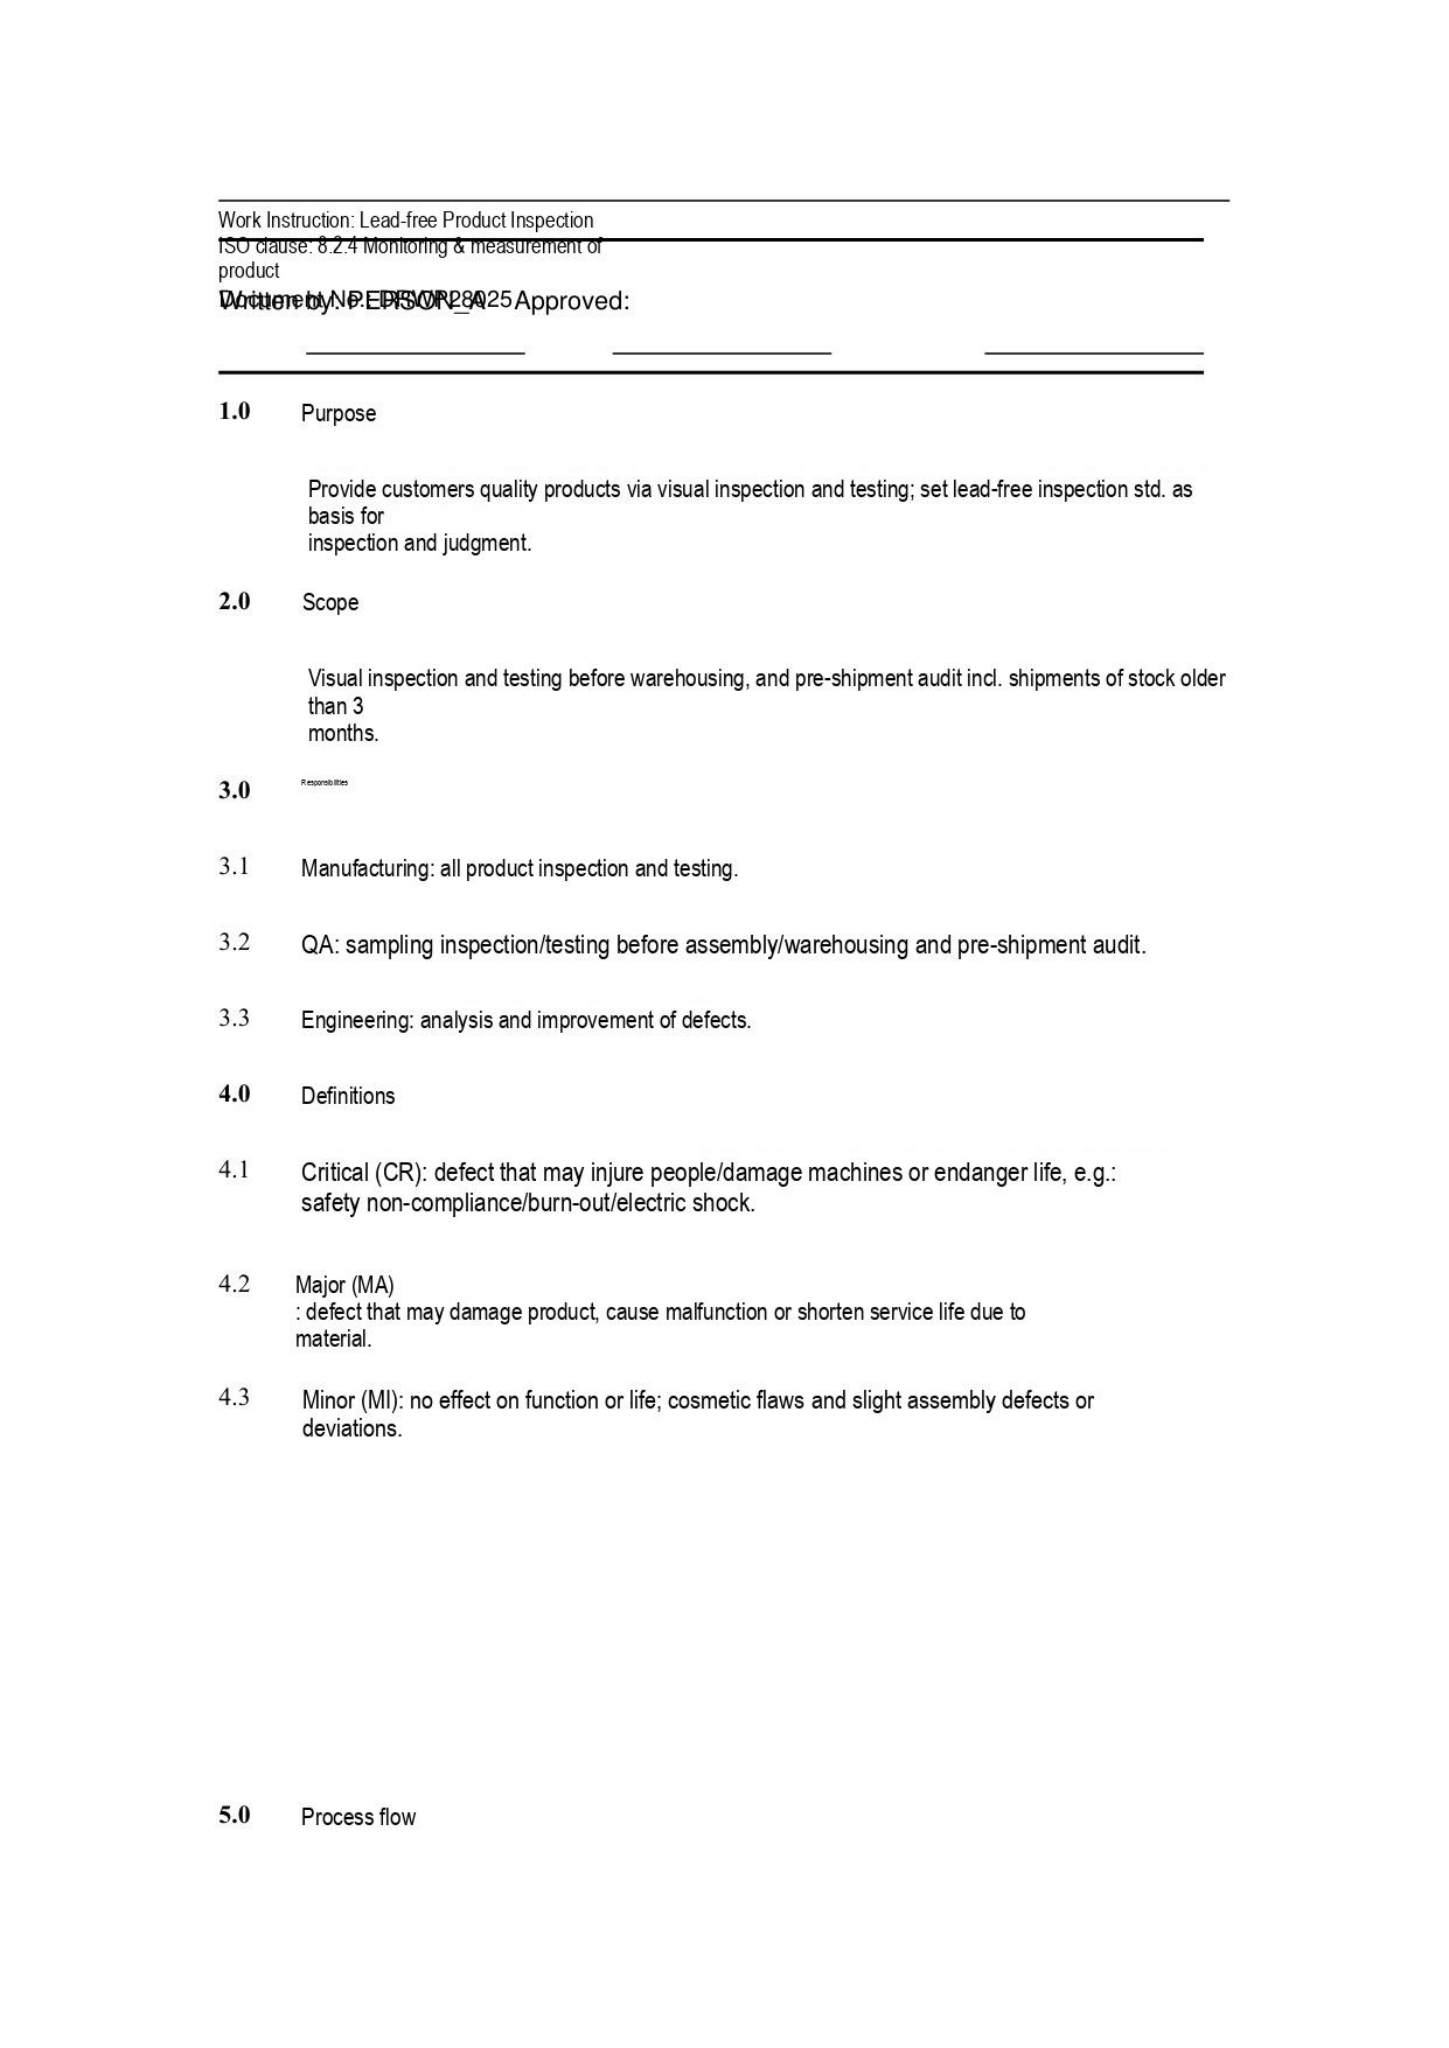Work Instruction: Lead-free Product Inspection
ISO clause: 8.2.4 Monitoring & measurement of product

Written by: PERSON_A Approved:

**1.0** Purpose

Provide customers quality products via visual inspection and testing; set lead-free inspection std. as basis for
inspection and judgment.

**2.0** Scope

Visual inspection and testing before warehousing, and pre-shipment audit incl. shipments of stock older than 3
months.

**3.0** Responsibilities

3.1 Manufacturing: all product inspection and testing.

3.2 QA: sampling inspection/testing before assembly/warehousing and pre-shipment audit.

3.3 Engineering: analysis and improvement of defects.

**4.0** Definitions

4.1 Critical (CR): defect that may injure people/damage machines or endanger life, e.g.:
safety non-compliance/burn-out/electric shock.

4.2 Major (MA)
: defect that may damage product, cause malfunction or shorten service life due to
material.

4.3 Minor (MI): no effect on function or life; cosmetic flaws and slight assembly defects or
deviations.

**5.0** Process flow
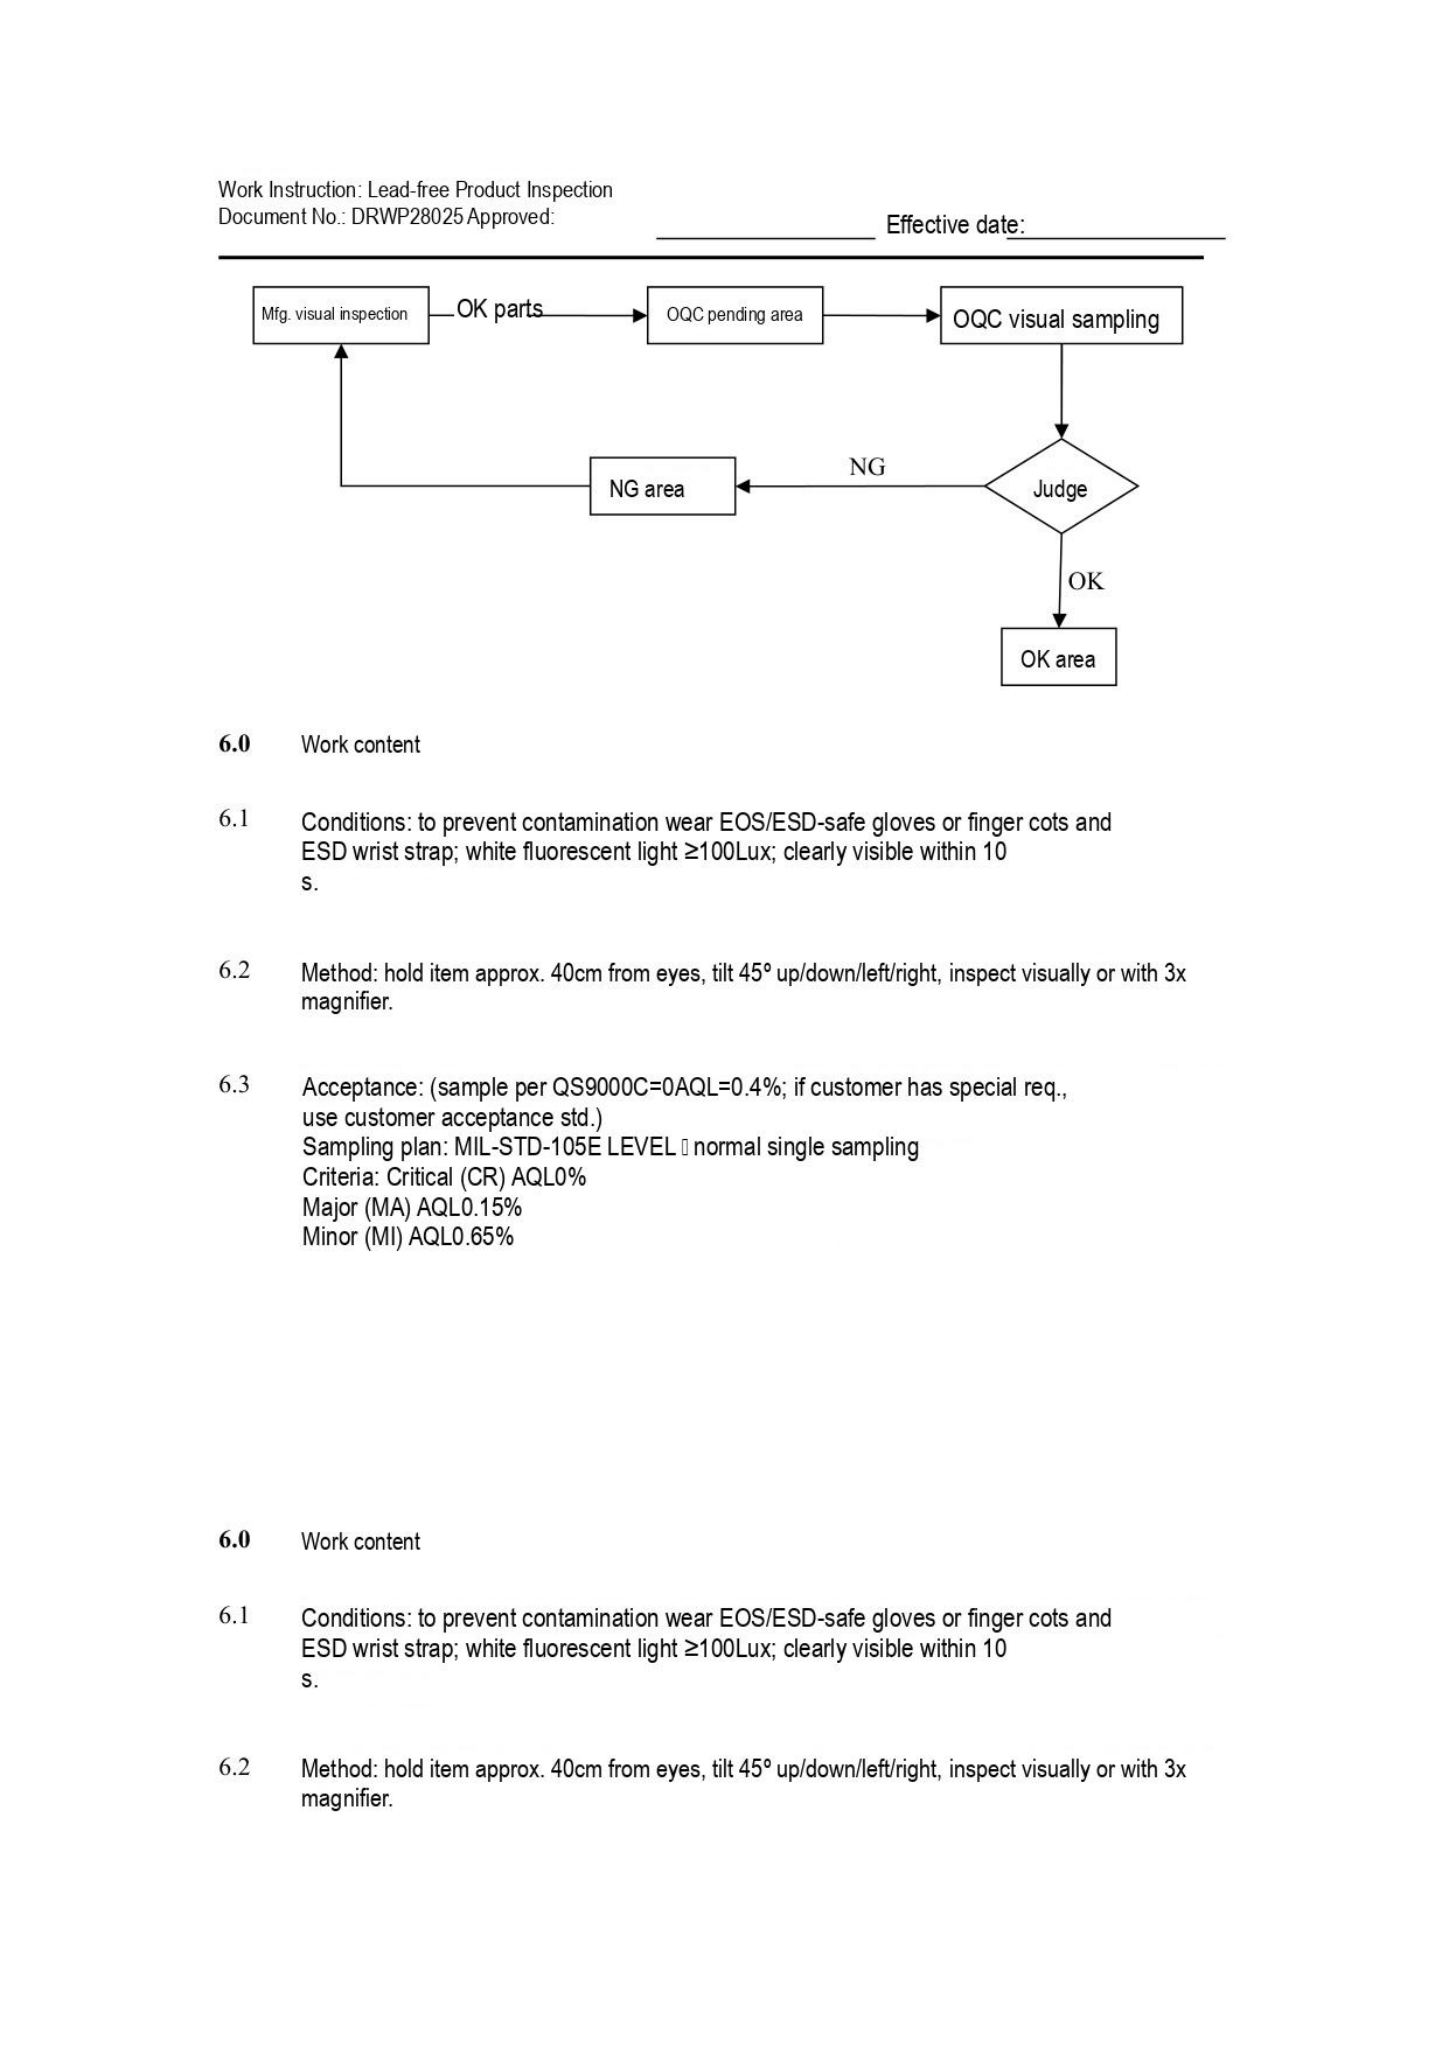Work Instruction: Lead-free Product Inspection
Document No.: DRWP28025 Approved: Effective date:

Mfg. visual inspection
OK parts
OQC pending area
OQC visual sampling
Judge
NG
NG area
OK
OK area

6.0 Work content

6.1 Conditions: to prevent contamination wear EOS/ESD-safe gloves or finger cots and ESD wrist strap; white fluorescent light ≥100Lux; clearly visible within 10 s.

6.2 Method: hold item approx. 40cm from eyes, tilt 45° up/down/left/right, inspect visually or with 3x magnifier.

6.3 Acceptance: (sample per QS9000C=0AQL=0.4%; if customer has special req., use customer acceptance std.)
Sampling plan: MIL-STD-105E LEVEL normal single sampling
Criteria: Critical (CR) AQL0%
Major (MA) AQL0.15%
Minor (MI) AQL0.65%

6.0 Work content

6.1 Conditions: to prevent contamination wear EOS/ESD-safe gloves or finger cots and ESD wrist strap; white fluorescent light ≥100Lux; clearly visible within 10 s.

6.2 Method: hold item approx. 40cm from eyes, tilt 45° up/down/left/right, inspect visually or with 3x magnifier.
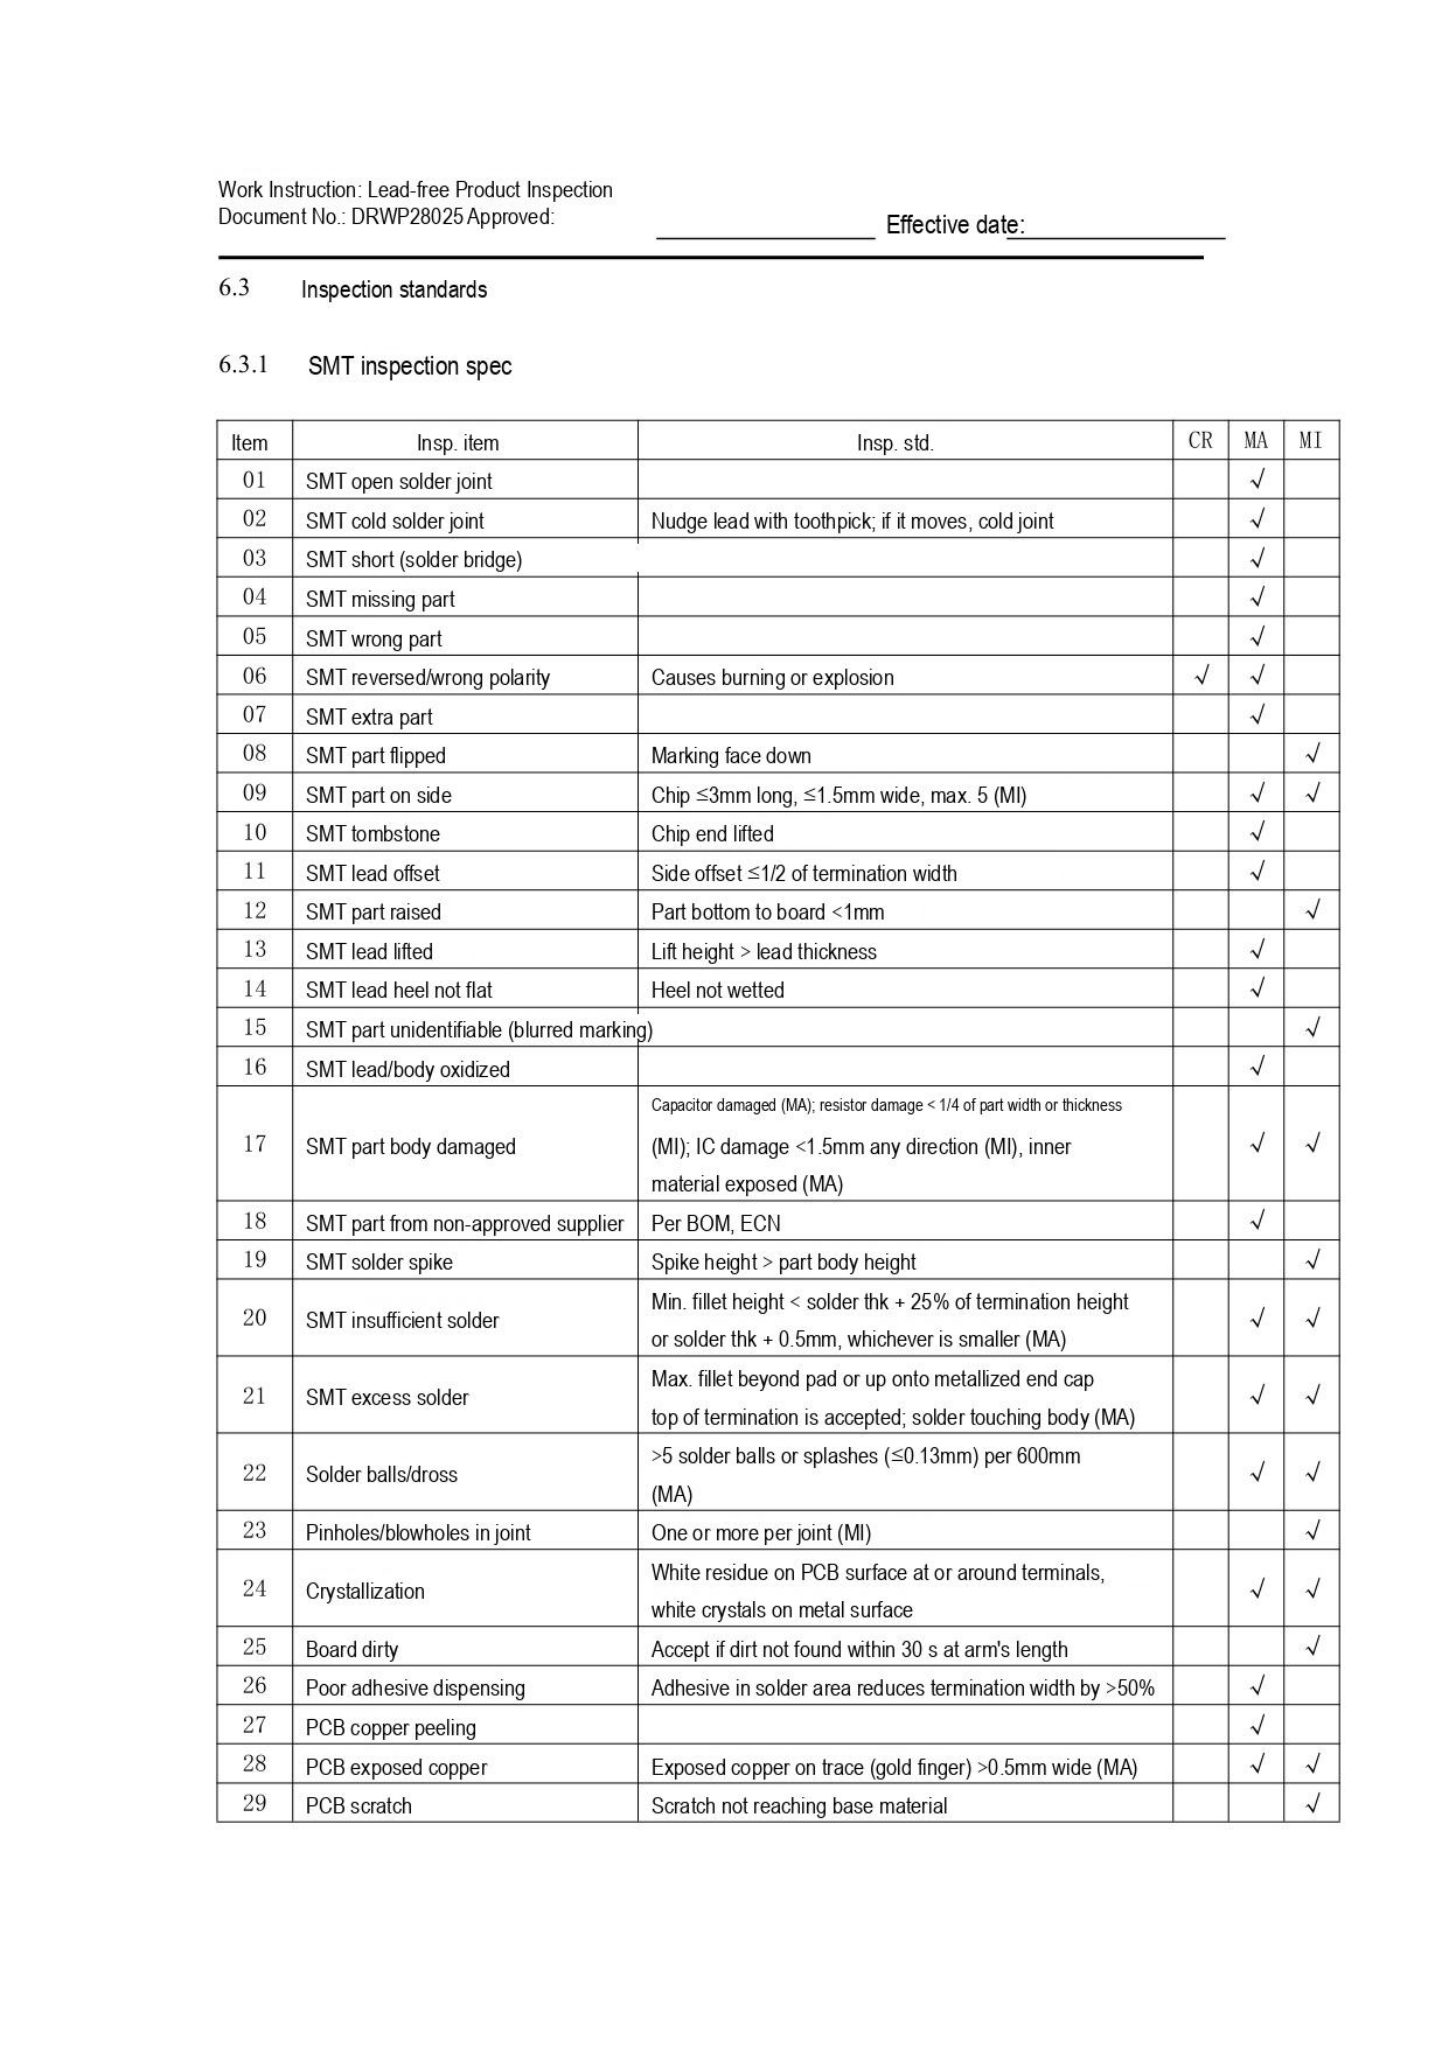Work Instruction: Lead-free Product Inspection
Document No.: DRWP28025 Approved: Effective date:

6.3 Inspection standards

6.3.1 SMT inspection spec

| Item | Insp. item | Insp. std. | CR | MA | MI |
|---|---|---|---|---|---|
| 01 | SMT open solder joint | | | √ | |
| 02 | SMT cold solder joint | Nudge lead with toothpick; if it moves, cold joint | | √ | |
| 03 | SMT short (solder bridge) | | | √ | |
| 04 | SMT missing part | | | √ | |
| 05 | SMT wrong part | | | √ | |
| 06 | SMT reversed/wrong polarity | Causes burning or explosion | √ | √ | |
| 07 | SMT extra part | | | √ | |
| 08 | SMT part flipped | Marking face down | | | √ |
| 09 | SMT part on side | Chip ≤3mm long, ≤1.5mm wide, max. 5 (MI) | | √ | √ |
| 10 | SMT tombstone | Chip end lifted | | √ | |
| 11 | SMT lead offset | Side offset ≤1/2 of termination width | | √ | |
| 12 | SMT part raised | Part bottom to board <1mm | | | √ |
| 13 | SMT lead lifted | Lift height > lead thickness | | √ | |
| 14 | SMT lead heel not flat | Heel not wetted | | √ | |
| 15 | SMT part unidentifiable (blurred marking) | | | | √ |
| 16 | SMT lead/body oxidized | | | √ | |
| 17 | SMT part body damaged | Capacitor damaged (MA); resistor damage < 1/4 of part width or thickness (MI); IC damage <1.5mm any direction (MI), inner material exposed (MA) | | √ | √ |
| 18 | SMT part from non-approved supplier | Per BOM, ECN | | √ | |
| 19 | SMT solder spike | Spike height > part body height | | | √ |
| 20 | SMT insufficient solder | Min. fillet height < solder thk + 25% of termination height or solder thk + 0.5mm, whichever is smaller (MA) | | √ | √ |
| 21 | SMT excess solder | Max. fillet beyond pad or up onto metallized end cap top of termination is accepted; solder touching body (MA) | | √ | √ |
| 22 | Solder balls/dross | >5 solder balls or splashes (≤0.13mm) per 600mm (MA) | | √ | √ |
| 23 | Pinholes/blowholes in joint | One or more per joint (MI) | | | √ |
| 24 | Crystallization | White residue on PCB surface at or around terminals, white crystals on metal surface | | √ | √ |
| 25 | Board dirty | Accept if dirt not found within 30 s at arm's length | | | √ |
| 26 | Poor adhesive dispensing | Adhesive in solder area reduces termination width by >50% | | √ | |
| 27 | PCB copper peeling | | | √ | |
| 28 | PCB exposed copper | Exposed copper on trace (gold finger) >0.5mm wide (MA) | | √ | √ |
| 29 | PCB scratch | Scratch not reaching base material | | | √ |
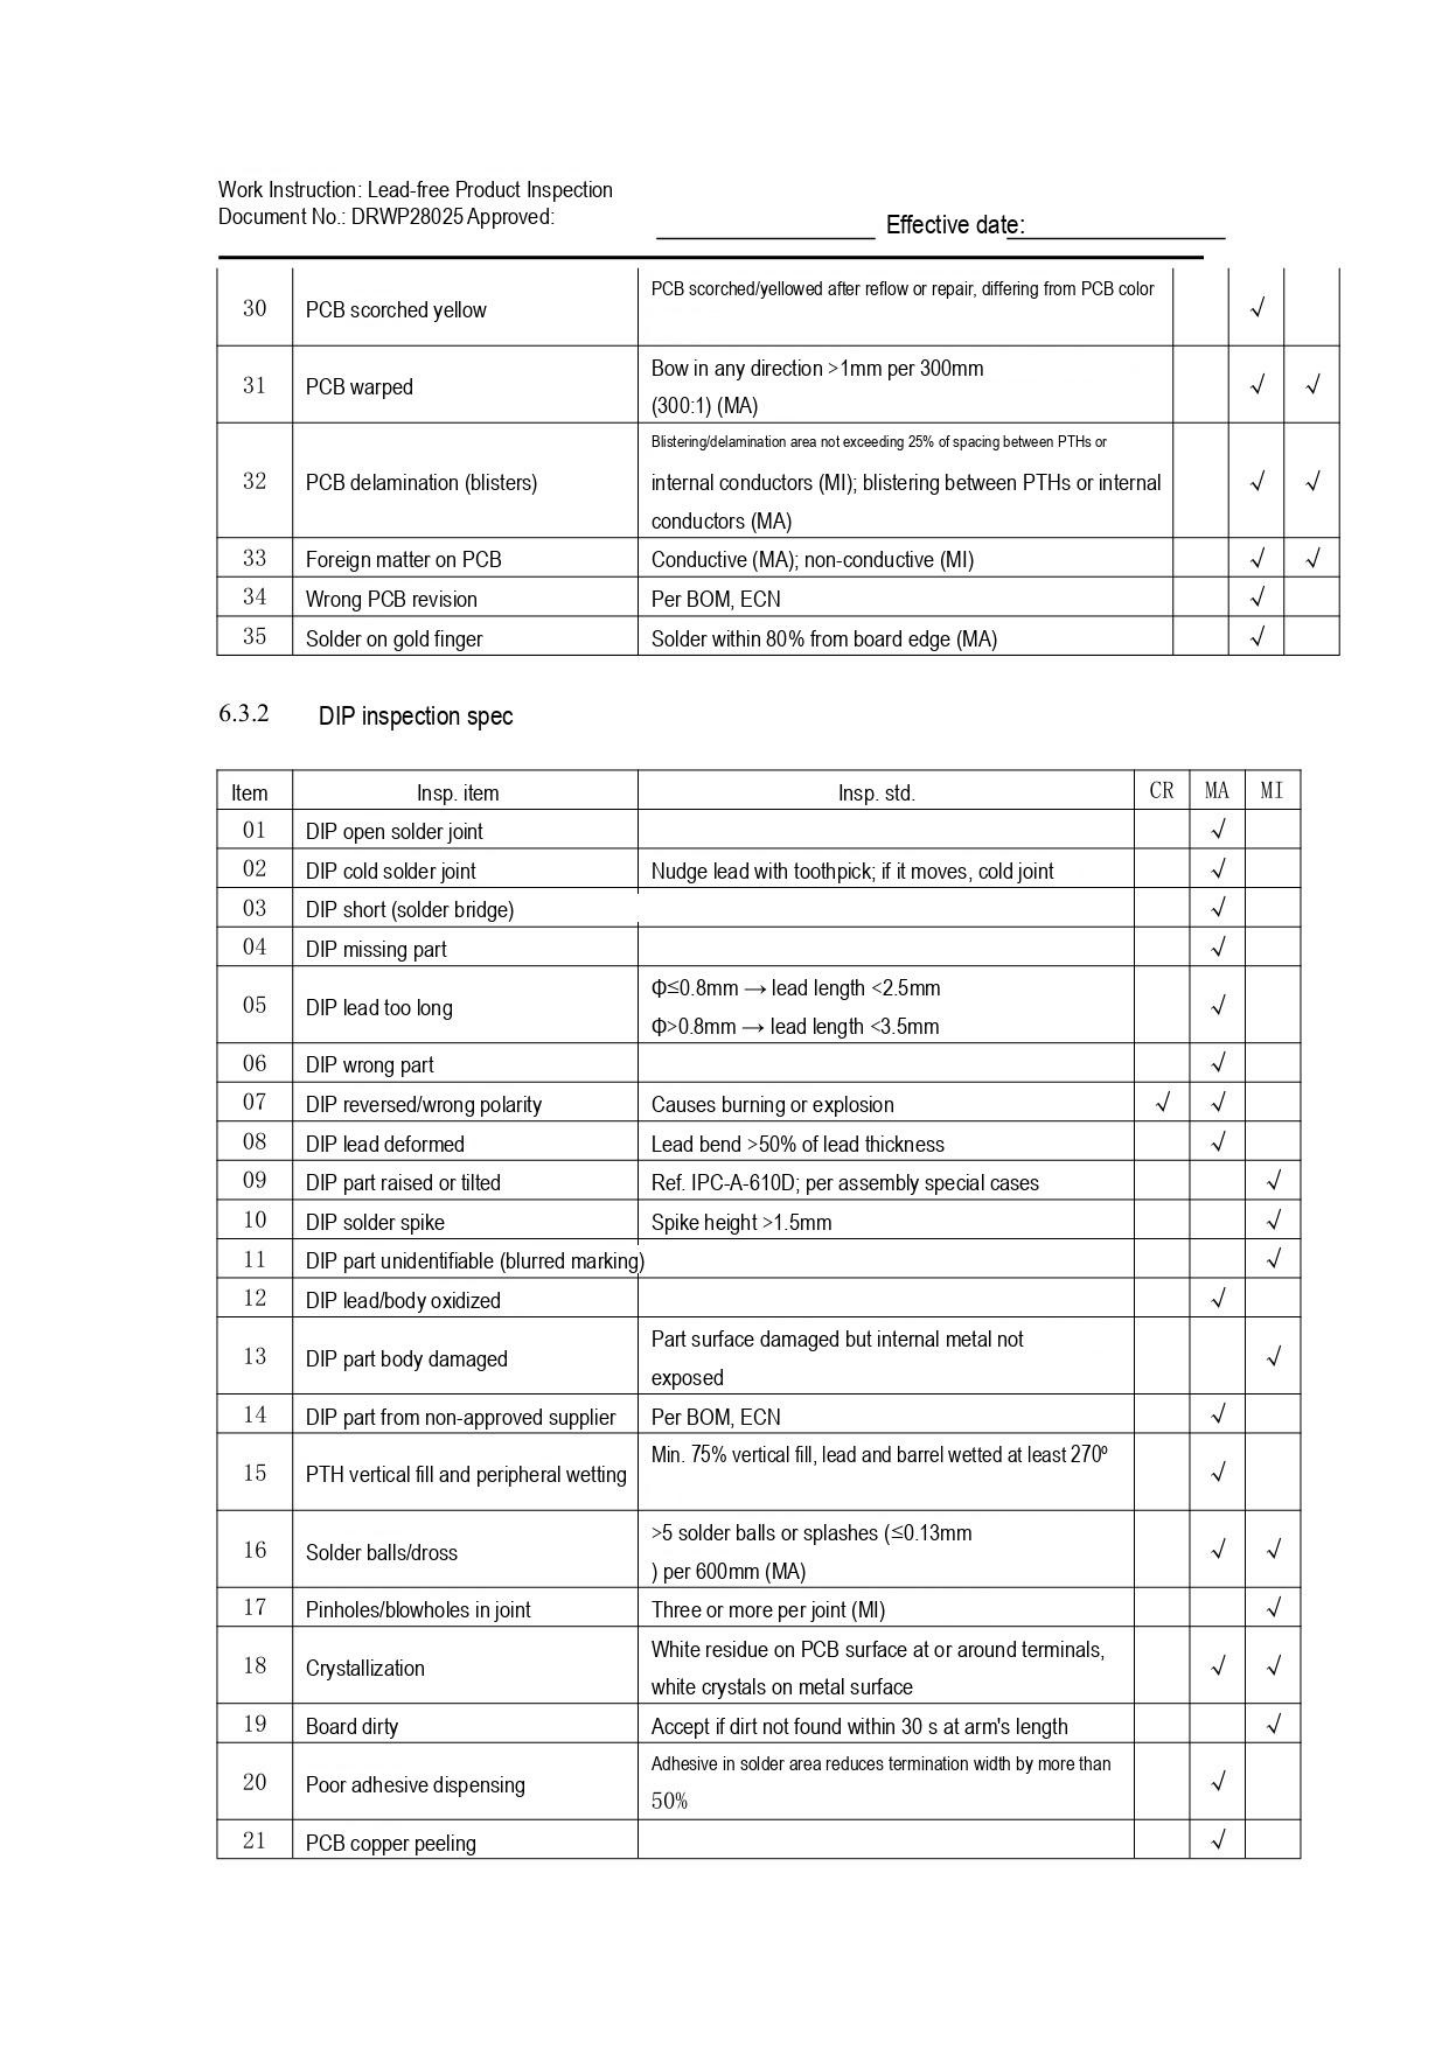Work Instruction: Lead-free Product Inspection
Document No.: DRWP28025 Approved: Effective date:

| | | | | | |
|---|---|---|---|---|---|
| 30 | PCB scorched yellow | PCB scorched/yellowed after reflow or repair, differing from PCB color | | √ | |
| 31 | PCB warped | Bow in any direction >1mm per 300mm (300:1) (MA) | | √ | √ |
| 32 | PCB delamination (blisters) | Blistering/delamination area not exceeding 25% of spacing between PTHs or internal conductors (MI); blistering between PTHs or internal conductors (MA) | | √ | √ |
| 33 | Foreign matter on PCB | Conductive (MA); non-conductive (MI) | | √ | √ |
| 34 | Wrong PCB revision | Per BOM, ECN | | √ | |
| 35 | Solder on gold finger | Solder within 80% from board edge (MA) | | √ | |

6.3.2 DIP inspection spec

| Item | Insp. item | Insp. std. | CR | MA | MI |
|---|---|---|---|---|---|
| 01 | DIP open solder joint | | | √ | |
| 02 | DIP cold solder joint | Nudge lead with toothpick; if it moves, cold joint | | √ | |
| 03 | DIP short (solder bridge) | | | √ | |
| 04 | DIP missing part | | | √ | |
| 05 | DIP lead too long | Φ≤0.8mm → lead length <2.5mm<br>Φ>0.8mm → lead length <3.5mm | | √ | |
| 06 | DIP wrong part | | | √ | |
| 07 | DIP reversed/wrong polarity | Causes burning or explosion | √ | √ | |
| 08 | DIP lead deformed | Lead bend >50% of lead thickness | | √ | |
| 09 | DIP part raised or tilted | Ref. IPC-A-610D; per assembly special cases | | | √ |
| 10 | DIP solder spike | Spike height >1.5mm | | | √ |
| 11 | DIP part unidentifiable (blurred marking) | | | | √ |
| 12 | DIP lead/body oxidized | | | √ | |
| 13 | DIP part body damaged | Part surface damaged but internal metal not exposed | | | √ |
| 14 | DIP part from non-approved supplier | Per BOM, ECN | | √ | |
| 15 | PTH vertical fill and peripheral wetting | Min. 75% vertical fill, lead and barrel wetted at least 270º | | √ | |
| 16 | Solder balls/dross | >5 solder balls or splashes (≤0.13mm ) per 600mm (MA) | | √ | √ |
| 17 | Pinholes/blowholes in joint | Three or more per joint (MI) | | | √ |
| 18 | Crystallization | White residue on PCB surface at or around terminals, white crystals on metal surface | | √ | √ |
| 19 | Board dirty | Accept if dirt not found within 30 s at arm's length | | | √ |
| 20 | Poor adhesive dispensing | Adhesive in solder area reduces termination width by more than 50% | | √ | |
| 21 | PCB copper peeling | | | √ | |
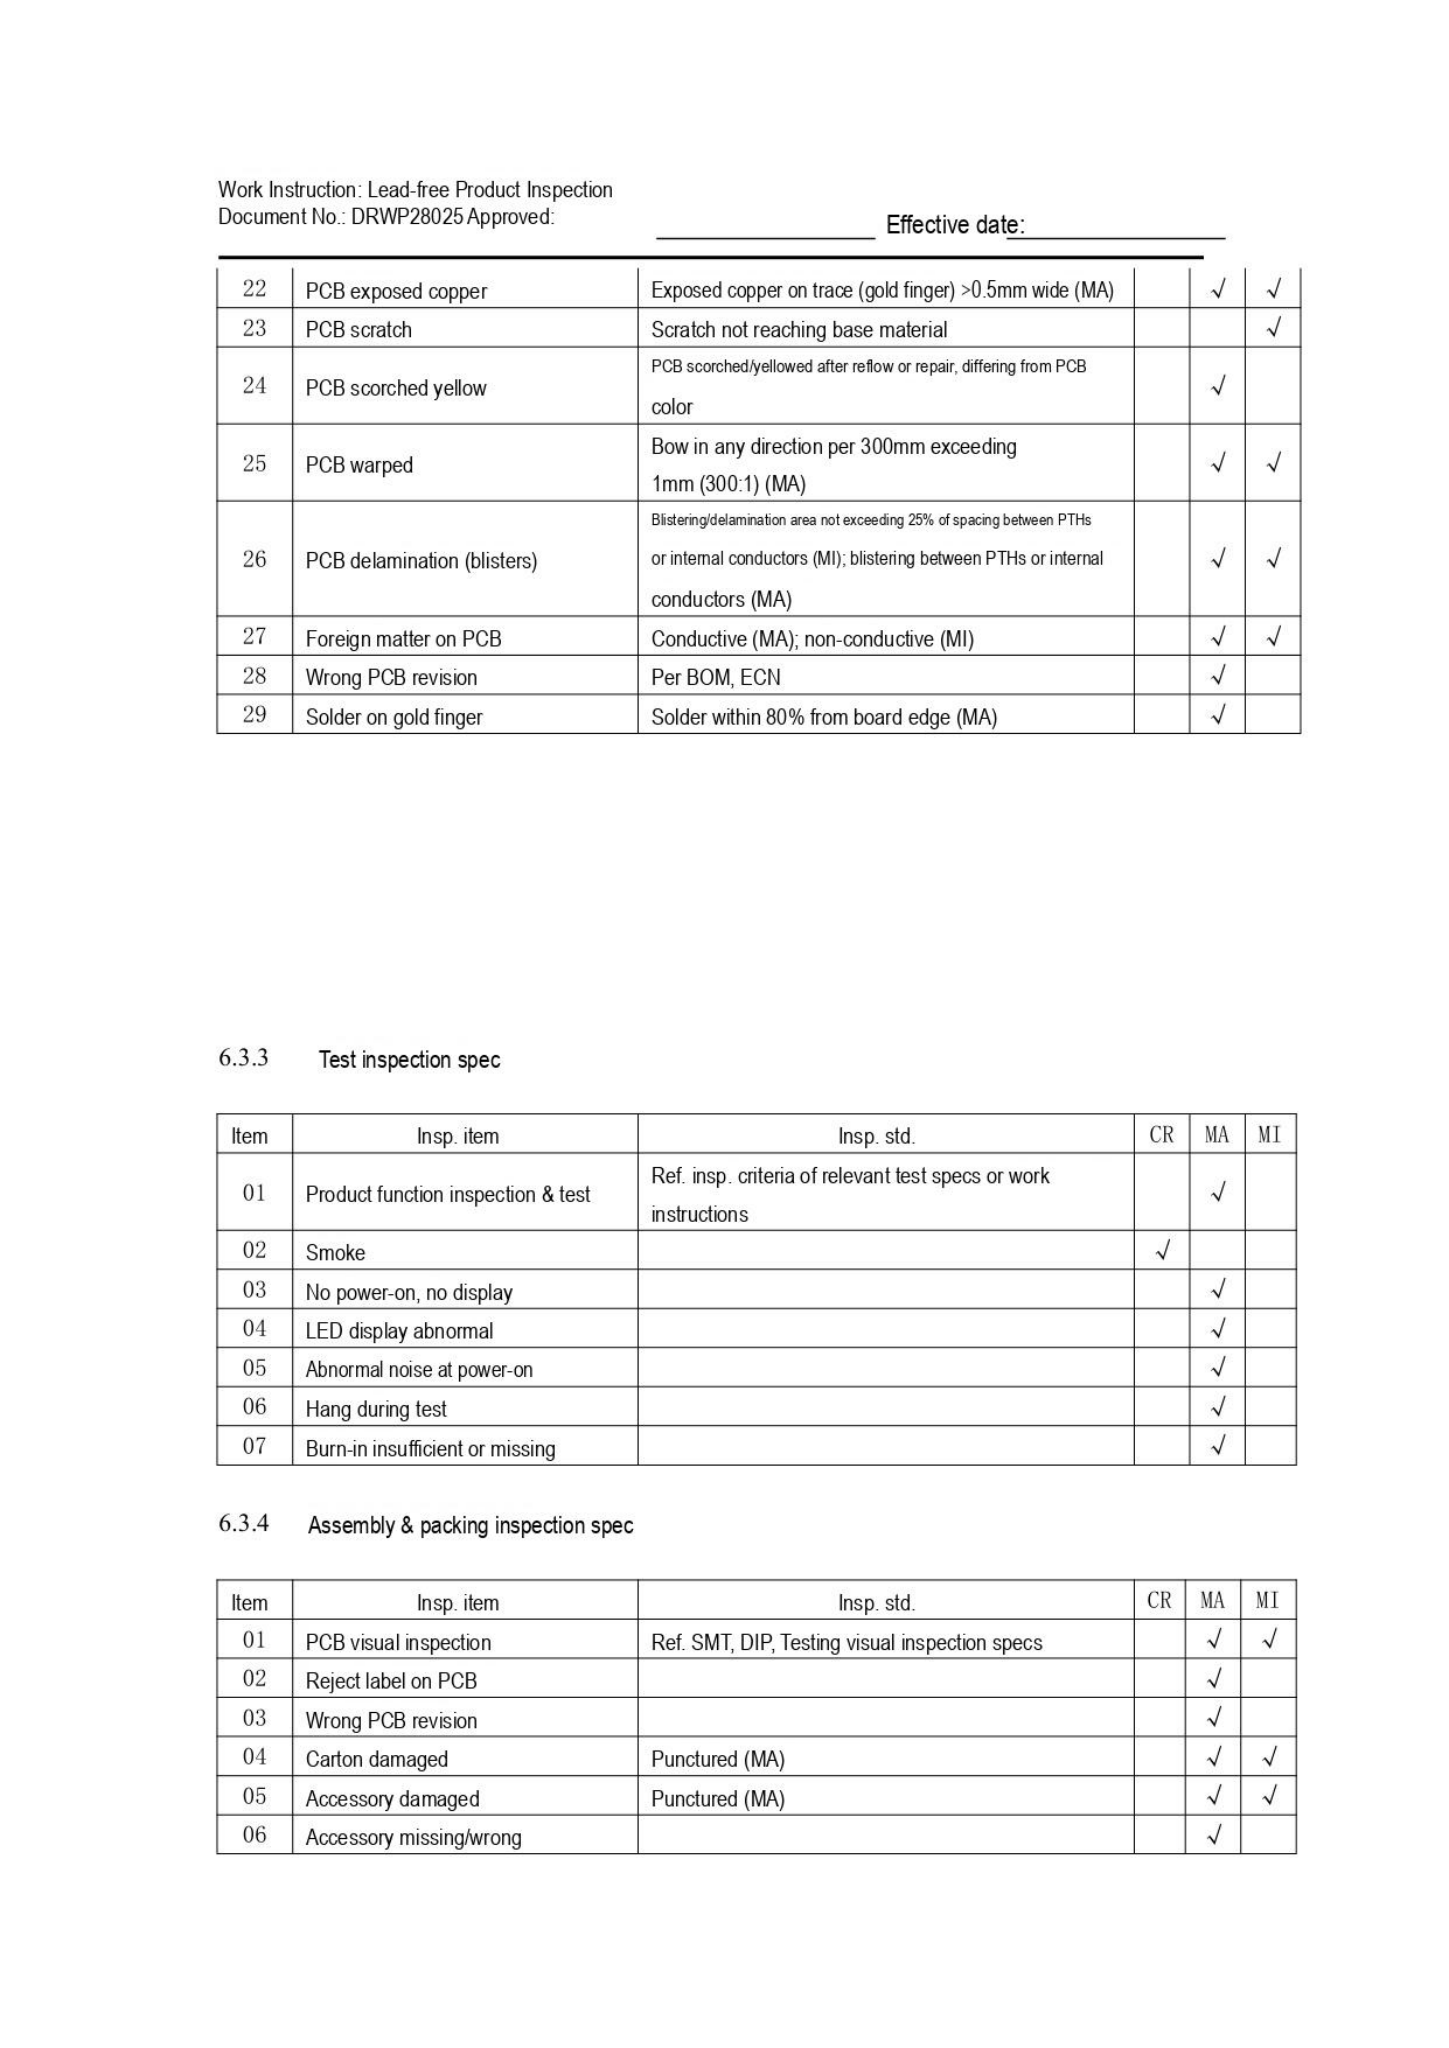Work Instruction: Lead-free Product Inspection
Document No.: DRWP28025 Approved: ____________ Effective date: ____________

| | | | | | |
|---|---|---|---|---|---|
| 22 | PCB exposed copper | Exposed copper on trace (gold finger) >0.5mm wide (MA) | | √ | √ |
| 23 | PCB scratch | Scratch not reaching base material | | | √ |
| 24 | PCB scorched yellow | PCB scorched/yellowed after reflow or repair, differing from PCB color | | √ | |
| 25 | PCB warped | Bow in any direction per 300mm exceeding 1mm (300:1) (MA) | | √ | √ |
| 26 | PCB delamination (blisters) | Blistering/delamination area not exceeding 25% of spacing between PTHs or internal conductors (MI); blistering between PTHs or internal conductors (MA) | | √ | √ |
| 27 | Foreign matter on PCB | Conductive (MA); non-conductive (MI) | | √ | √ |
| 28 | Wrong PCB revision | Per BOM, ECN | | √ | |
| 29 | Solder on gold finger | Solder within 80% from board edge (MA) | | √ | |

6.3.3 Test inspection spec

| Item | Insp. item | Insp. std. | CR | MA | MI |
|---|---|---|---|---|---|
| 01 | Product function inspection & test | Ref. insp. criteria of relevant test specs or work instructions | | √ | |
| 02 | Smoke | | √ | | |
| 03 | No power-on, no display | | | √ | |
| 04 | LED display abnormal | | | √ | |
| 05 | Abnormal noise at power-on | | | √ | |
| 06 | Hang during test | | | √ | |
| 07 | Burn-in insufficient or missing | | | √ | |

6.3.4 Assembly & packing inspection spec

| Item | Insp. item | Insp. std. | CR | MA | MI |
|---|---|---|---|---|---|
| 01 | PCB visual inspection | Ref. SMT, DIP, Testing visual inspection specs | | √ | √ |
| 02 | Reject label on PCB | | | √ | |
| 03 | Wrong PCB revision | | | √ | |
| 04 | Carton damaged | Punctured (MA) | | √ | √ |
| 05 | Accessory damaged | Punctured (MA) | | √ | √ |
| 06 | Accessory missing/wrong | | | √ | |
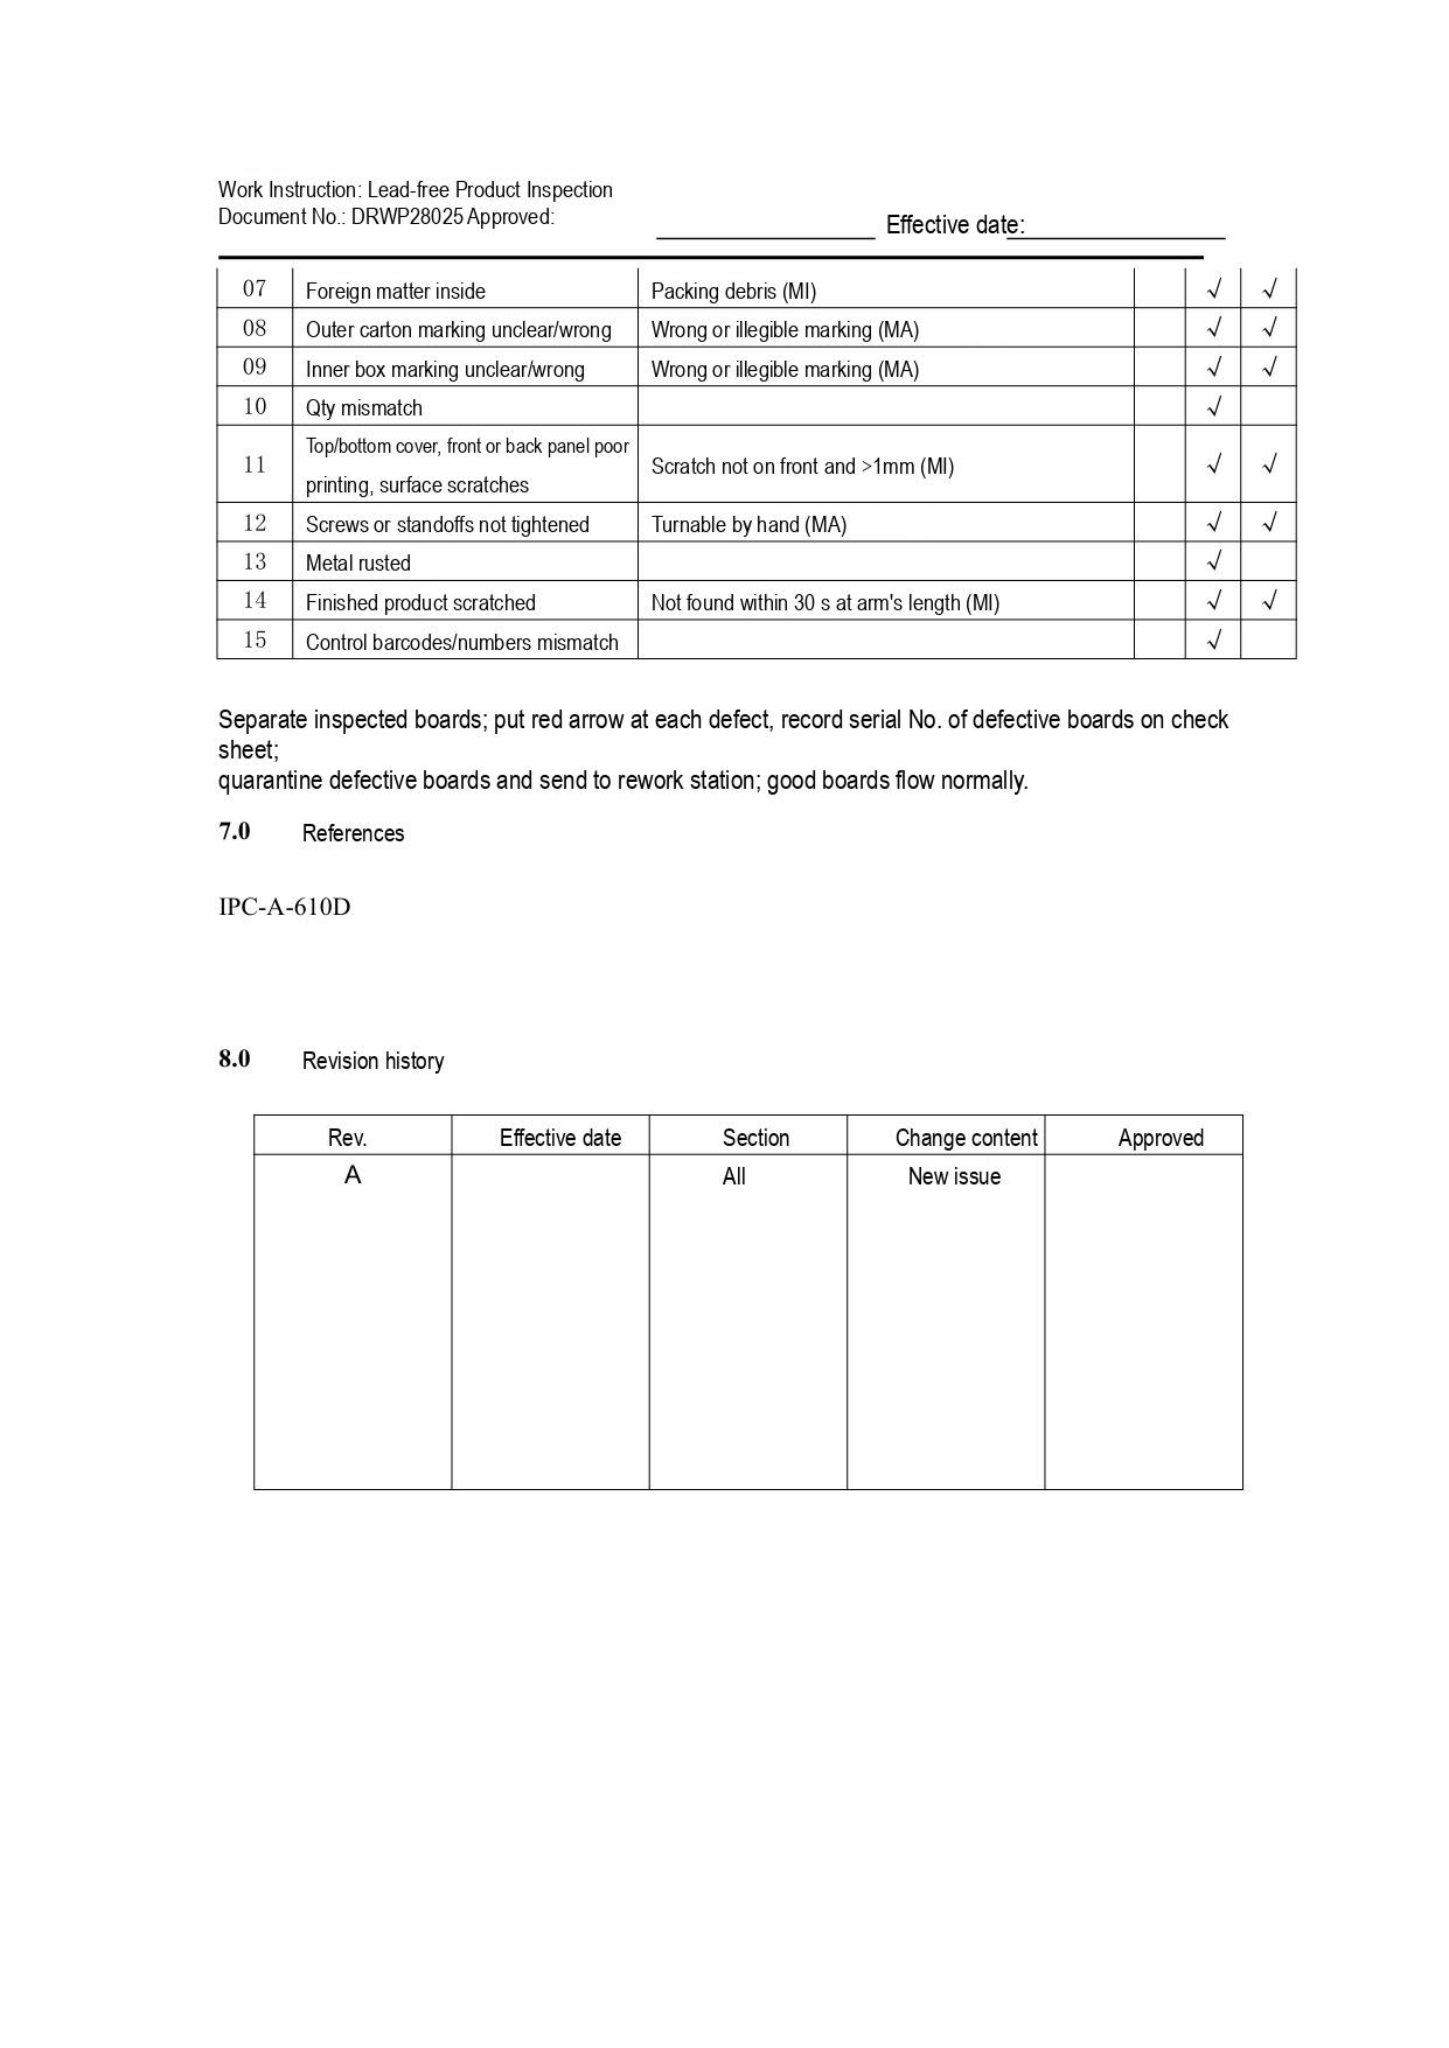Work Instruction: Lead-free Product Inspection
Document No.: DRWP28025 Approved: Effective date:

| | | | | | |
|---|---|---|---|---|---|
| 07 | Foreign matter inside | Packing debris (MI) | | √ | √ |
| 08 | Outer carton marking unclear/wrong | Wrong or illegible marking (MA) | | √ | √ |
| 09 | Inner box marking unclear/wrong | Wrong or illegible marking (MA) | | √ | √ |
| 10 | Qty mismatch | | | √ | |
| 11 | Top/bottom cover, front or back panel poor printing, surface scratches | Scratch not on front and >1mm (MI) | | √ | √ |
| 12 | Screws or standoffs not tightened | Turnable by hand (MA) | | √ | √ |
| 13 | Metal rusted | | | √ | |
| 14 | Finished product scratched | Not found within 30 s at arm's length (MI) | | √ | √ |
| 15 | Control barcodes/numbers mismatch | | | √ | |

Separate inspected boards; put red arrow at each defect, record serial No. of defective boards on check sheet;
quarantine defective boards and send to rework station; good boards flow normally.

7.0 References

IPC-A-610D

8.0 Revision history

| Rev. | Effective date | Section | Change content | Approved |
|---|---|---|---|---|
| A | | All | New issue | |